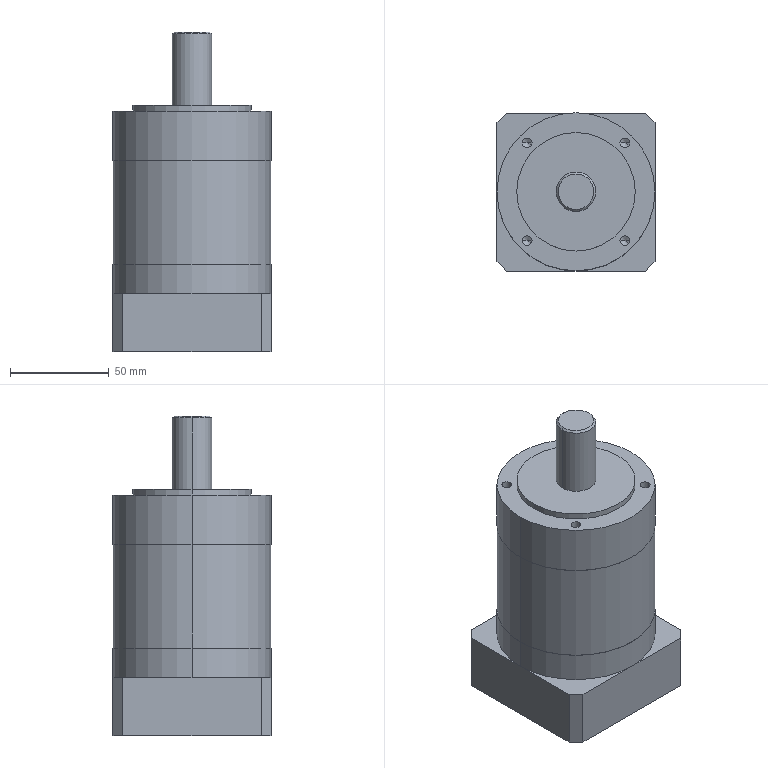Part | STEP file | PL80-40 | 1 solid | 68 faces | box 80 x 80 x 162 mm | volume 651730 mm3 | cylinder 30 | plane 20 | cone 18 | commonest cylinder face diameters 5 x16 80 x4 16 x2 20 x2 60 x2 70 x2